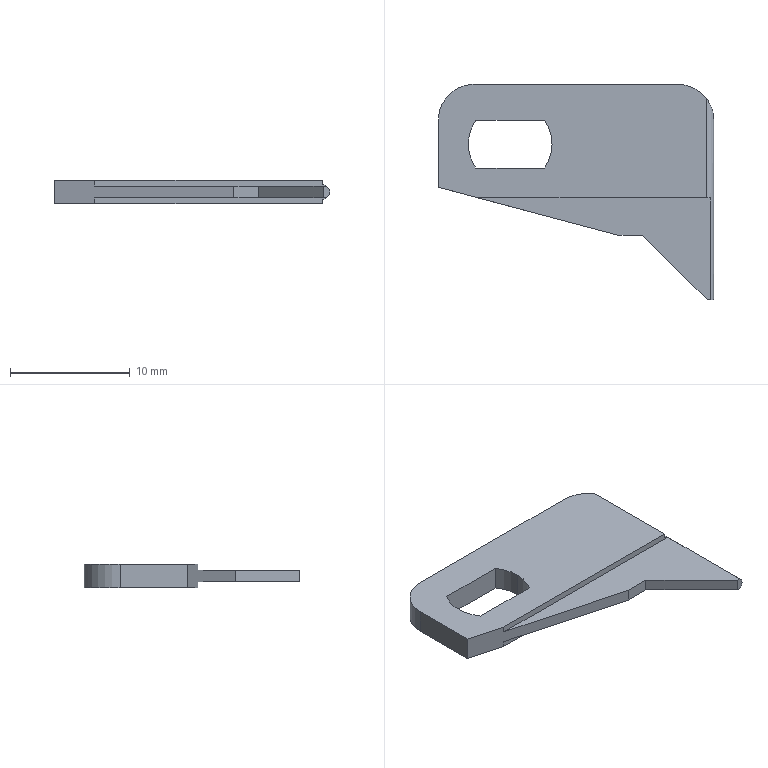Part | NX | 1 solid | 23 faces | box 23 x 18 x 2 mm | volume 428.306 mm3 | plane 16 | cylinder 7 | commonest cylinder face diameters 7 x3 1.2 x2 6 x2
STEP:
#1=CARTESIAN_POINT('',(16.4,3.8,0.));
#2=VERTEX_POINT('',#1);
#3=CARTESIAN_POINT('',(16.4,-4.5,0.));
#4=VERTEX_POINT('',#3);
#5=CARTESIAN_POINT('',(16.4,3.8,0.));
#6=DIRECTION('',(0.,-1.,0.));
#7=VECTOR('',#6,1000.);
#8=LINE('',#5,#7);
#9=EDGE_CURVE('',#2,#4,#8,.T.);
#10=ORIENTED_EDGE('',*,*,#9,.T.);
#11=CARTESIAN_POINT('',(-2.625,-4.5,0.));
#12=VERTEX_POINT('',#11);
#13=CARTESIAN_POINT('',(16.4,-4.5,0.));
#14=DIRECTION('',(-1.,0.,0.));
#15=VECTOR('',#14,1000.);
#16=LINE('',#13,#15);
#17=EDGE_CURVE('',#4,#12,#16,.T.);
#18=ORIENTED_EDGE('',*,*,#17,.T.);
#19=CARTESIAN_POINT('',(-6.,-3.6,0.));
#20=VERTEX_POINT('',#19);
#21=CARTESIAN_POINT('',(-6.,-3.6,0.));
#22=DIRECTION('',(0.9662,-0.2577,0.));
#23=VECTOR('',#22,1000.);
#24=LINE('',#21,#23);
#25=EDGE_CURVE('',#20,#12,#24,.T.);
#26=ORIENTED_EDGE('',*,*,#25,.F.);
#27=CARTESIAN_POINT('',(-6.,2.,0.));
#28=VERTEX_POINT('',#27);
#29=CARTESIAN_POINT('',(-6.,-3.6,0.));
#30=DIRECTION('',(0.,1.,0.));
#31=VECTOR('',#30,1000.);
#32=LINE('',#29,#31);
#33=EDGE_CURVE('',#20,#28,#32,.T.);
#34=ORIENTED_EDGE('',*,*,#33,.T.);
#35=CARTESIAN_POINT('',(-3.,5.,0.));
#36=VERTEX_POINT('',#35);
#37=CARTESIAN_POINT('',(-3.,2.,0.));
#38=DIRECTION('',(0.,0.,1.));
#39=DIRECTION('',(0.,1.,0.));
#40=AXIS2_PLACEMENT_3D('',#37,#38,#39);
#41=CIRCLE('',#40,3.);
#42=EDGE_CURVE('',#36,#28,#41,.T.);
#43=ORIENTED_EDGE('',*,*,#42,.F.);
#44=CARTESIAN_POINT('',(14.,5.,0.));
#45=VERTEX_POINT('',#44);
#46=CARTESIAN_POINT('',(-3.,5.,0.));
#47=DIRECTION('',(1.,0.,0.));
#48=VECTOR('',#47,1000.);
#49=LINE('',#46,#48);
#50=EDGE_CURVE('',#36,#45,#49,.T.);
#51=ORIENTED_EDGE('',*,*,#50,.T.);
#52=CARTESIAN_POINT('',(14.,2.,0.));
#53=DIRECTION('',(0.,0.,1.));
#54=DIRECTION('',(0.8,0.6,0.));
#55=AXIS2_PLACEMENT_3D('',#52,#53,#54);
#56=CIRCLE('',#55,3.);
#57=EDGE_CURVE('',#2,#45,#56,.T.);
#58=ORIENTED_EDGE('',*,*,#57,.F.);
#59=EDGE_LOOP('',(#10,#18,#26,#34,#43,#51,#58));
#60=FACE_BOUND('',#59,.T.);
#61=CARTESIAN_POINT('',(-2.872,-2.,0.));
#62=VERTEX_POINT('',#61);
#63=CARTESIAN_POINT('',(-2.872,2.,0.));
#64=VERTEX_POINT('',#63);
#65=CARTESIAN_POINT('',(0.,0.,0.));
#66=DIRECTION('',(0.,0.,-1.));
#67=DIRECTION('',(-1.,0.,0.));
#68=AXIS2_PLACEMENT_3D('',#65,#66,#67);
#69=CIRCLE('',#68,3.5);
#70=EDGE_CURVE('',#62,#64,#69,.T.);
#71=ORIENTED_EDGE('',*,*,#70,.F.);
#72=CARTESIAN_POINT('',(2.872,-2.,0.));
#73=VERTEX_POINT('',#72);
#74=CARTESIAN_POINT('',(-2.872,-2.,0.));
#75=DIRECTION('',(1.,0.,0.));
#76=VECTOR('',#75,1000.);
#77=LINE('',#74,#76);
#78=EDGE_CURVE('',#62,#73,#77,.T.);
#79=ORIENTED_EDGE('',*,*,#78,.T.);
#80=CARTESIAN_POINT('',(3.5,0.,0.));
#81=VERTEX_POINT('',#80);
#82=CARTESIAN_POINT('',(0.,0.,0.));
#83=DIRECTION('',(0.,0.,-1.));
#84=DIRECTION('',(1.,0.,0.));
#85=AXIS2_PLACEMENT_3D('',#82,#83,#84);
#86=CIRCLE('',#85,3.5);
#87=EDGE_CURVE('',#81,#73,#86,.T.);
#88=ORIENTED_EDGE('',*,*,#87,.F.);
#89=CARTESIAN_POINT('',(2.872,2.,0.));
#90=VERTEX_POINT('',#89);
#91=CARTESIAN_POINT('',(0.,0.,0.));
#92=DIRECTION('',(0.,0.,-1.));
#93=DIRECTION('',(1.,0.,0.));
#94=AXIS2_PLACEMENT_3D('',#91,#92,#93);
#95=CIRCLE('',#94,3.5);
#96=EDGE_CURVE('',#90,#81,#95,.T.);
#97=ORIENTED_EDGE('',*,*,#96,.F.);
#98=CARTESIAN_POINT('',(2.872,2.,0.));
#99=DIRECTION('',(-1.,0.,0.));
#100=VECTOR('',#99,1000.);
#101=LINE('',#98,#100);
#102=EDGE_CURVE('',#90,#64,#101,.T.);
#103=ORIENTED_EDGE('',*,*,#102,.T.);
#104=EDGE_LOOP('',(#71,#79,#88,#97,#103));
#105=FACE_BOUND('',#104,.T.);
#106=CARTESIAN_POINT('',(0.,0.,0.));
#107=DIRECTION('',(0.,0.,1.));
#108=DIRECTION('',(1.,0.,0.));
#109=AXIS2_PLACEMENT_3D('',#106,#107,#108);
#110=PLANE('',#109);
#111=ADVANCED_FACE('',(#60,#105),#110,.F.);
#112=ORIENTED_EDGE('',*,*,#9,.F.);
#113=CARTESIAN_POINT('',(16.4,3.8,0.4));
#114=VERTEX_POINT('',#113);
#115=CARTESIAN_POINT('',(16.4,3.8,0.));
#116=DIRECTION('',(0.,0.,1.));
#117=VECTOR('',#116,1000.);
#118=LINE('',#115,#117);
#119=EDGE_CURVE('',#2,#114,#118,.T.);
#120=ORIENTED_EDGE('',*,*,#119,.T.);
#121=CARTESIAN_POINT('',(16.4,-4.5,0.4));
#122=VERTEX_POINT('',#121);
#123=CARTESIAN_POINT('',(16.4,3.8,0.4));
#124=DIRECTION('',(0.,-1.,0.));
#125=VECTOR('',#124,1000.);
#126=LINE('',#123,#125);
#127=EDGE_CURVE('',#114,#122,#126,.T.);
#128=ORIENTED_EDGE('',*,*,#127,.T.);
#129=CARTESIAN_POINT('',(16.4,-4.5,0.4));
#130=DIRECTION('',(0.,0.,-1.));
#131=VECTOR('',#130,1000.);
#132=LINE('',#129,#131);
#133=EDGE_CURVE('',#122,#4,#132,.T.);
#134=ORIENTED_EDGE('',*,*,#133,.T.);
#135=EDGE_LOOP('',(#112,#120,#128,#134));
#136=FACE_BOUND('',#135,.T.);
#137=CARTESIAN_POINT('',(16.4,-13.,0.4));
#138=DIRECTION('',(-1.,0.,0.));
#139=DIRECTION('',(0.,0.,1.));
#140=AXIS2_PLACEMENT_3D('',#137,#138,#139);
#141=PLANE('',#140);
#142=ADVANCED_FACE('',(#136),#141,.F.);
#143=CARTESIAN_POINT('',(16.732,-4.5,0.5));
#144=VERTEX_POINT('',#143);
#145=CARTESIAN_POINT('',(-2.625,-4.5,0.5));
#146=VERTEX_POINT('',#145);
#147=CARTESIAN_POINT('',(16.732,-4.5,0.5));
#148=DIRECTION('',(-1.,0.,0.));
#149=VECTOR('',#148,1000.);
#150=LINE('',#147,#149);
#151=EDGE_CURVE('',#144,#146,#150,.T.);
#152=ORIENTED_EDGE('',*,*,#151,.T.);
#153=CARTESIAN_POINT('',(-2.625,-4.5,0.5));
#154=DIRECTION('',(0.,0.,-1.));
#155=VECTOR('',#154,1000.);
#156=LINE('',#153,#155);
#157=EDGE_CURVE('',#146,#12,#156,.T.);
#158=ORIENTED_EDGE('',*,*,#157,.T.);
#159=ORIENTED_EDGE('',*,*,#17,.F.);
#160=ORIENTED_EDGE('',*,*,#133,.F.);
#161=CARTESIAN_POINT('',(16.4,-4.5,1.));
#162=DIRECTION('',(0.,1.,0.));
#163=DIRECTION('',(0.5528,0.,-0.8333));
#164=AXIS2_PLACEMENT_3D('',#161,#162,#163);
#165=CIRCLE('',#164,0.6);
#166=EDGE_CURVE('',#144,#122,#165,.T.);
#167=ORIENTED_EDGE('',*,*,#166,.F.);
#168=EDGE_LOOP('',(#152,#158,#159,#160,#167));
#169=FACE_BOUND('',#168,.T.);
#170=CARTESIAN_POINT('',(-6.,-4.5,0.5));
#171=DIRECTION('',(0.,1.,0.));
#172=DIRECTION('',(1.,0.,0.));
#173=AXIS2_PLACEMENT_3D('',#170,#171,#172);
#174=PLANE('',#173);
#175=ADVANCED_FACE('',(#169),#174,.F.);
#176=CARTESIAN_POINT('',(16.732,-13.,0.5));
#177=VERTEX_POINT('',#176);
#178=CARTESIAN_POINT('',(16.732,-4.5,0.5));
#179=DIRECTION('',(0.,-1.,0.));
#180=VECTOR('',#179,1000.);
#181=LINE('',#178,#180);
#182=EDGE_CURVE('',#144,#177,#181,.T.);
#183=ORIENTED_EDGE('',*,*,#182,.T.);
#184=CARTESIAN_POINT('',(16.45,-13.,0.5));
#185=VERTEX_POINT('',#184);
#186=CARTESIAN_POINT('',(16.732,-13.,0.5));
#187=DIRECTION('',(-1.,0.,0.));
#188=VECTOR('',#187,1000.);
#189=LINE('',#186,#188);
#190=EDGE_CURVE('',#177,#185,#189,.T.);
#191=ORIENTED_EDGE('',*,*,#190,.T.);
#192=CARTESIAN_POINT('',(11.05,-7.6,0.5));
#193=VERTEX_POINT('',#192);
#194=CARTESIAN_POINT('',(11.05,-7.6,0.5));
#195=DIRECTION('',(0.7071,-0.7071,0.));
#196=VECTOR('',#195,1000.);
#197=LINE('',#194,#196);
#198=EDGE_CURVE('',#193,#185,#197,.T.);
#199=ORIENTED_EDGE('',*,*,#198,.F.);
#200=CARTESIAN_POINT('',(9.,-7.6,0.5));
#201=VERTEX_POINT('',#200);
#202=CARTESIAN_POINT('',(11.05,-7.6,0.5));
#203=DIRECTION('',(-1.,0.,0.));
#204=VECTOR('',#203,1000.);
#205=LINE('',#202,#204);
#206=EDGE_CURVE('',#193,#201,#205,.T.);
#207=ORIENTED_EDGE('',*,*,#206,.T.);
#208=CARTESIAN_POINT('',(-2.625,-4.5,0.5));
#209=DIRECTION('',(0.9662,-0.2577,0.));
#210=VECTOR('',#209,1000.);
#211=LINE('',#208,#210);
#212=EDGE_CURVE('',#146,#201,#211,.T.);
#213=ORIENTED_EDGE('',*,*,#212,.F.);
#214=ORIENTED_EDGE('',*,*,#151,.F.);
#215=EDGE_LOOP('',(#183,#191,#199,#207,#213,#214));
#216=FACE_BOUND('',#215,.T.);
#217=CARTESIAN_POINT('',(-6.,-13.,0.5));
#218=DIRECTION('',(0.,0.,1.));
#219=DIRECTION('',(1.,0.,0.));
#220=AXIS2_PLACEMENT_3D('',#217,#218,#219);
#221=PLANE('',#220);
#222=ADVANCED_FACE('',(#216),#221,.F.);
#223=CARTESIAN_POINT('',(17.,2.,1.));
#224=VERTEX_POINT('',#223);
#225=CARTESIAN_POINT('',(17.,-13.,1.));
#226=VERTEX_POINT('',#225);
#227=CARTESIAN_POINT('',(17.,-13.,1.));
#228=DIRECTION('',(0.,-1.,0.));
#229=VECTOR('',#228,1000.);
#230=LINE('',#227,#229);
#231=EDGE_CURVE('',#224,#226,#230,.T.);
#232=ORIENTED_EDGE('',*,*,#231,.F.);
#233=CARTESIAN_POINT('',(16.4,3.8,1.6));
#234=VERTEX_POINT('',#233);
#235=CARTESIAN_POINT('',(17.,2.,1.));
#236=CARTESIAN_POINT('',(17.,2.241,1.108));
#237=CARTESIAN_POINT('',(16.937,2.669,1.297));
#238=CARTESIAN_POINT('',(16.788,3.166,1.49));
#239=CARTESIAN_POINT('',(16.542,3.61,1.6));
#240=CARTESIAN_POINT('',(16.4,3.8,1.6));
#241=B_SPLINE_CURVE_WITH_KNOTS('',3,(#235,#236,#237,#238,#239,#240),.UNSPECIFIED.,.F.,.F.,(4,1,1,4),(0.,0.25,0.5,1.),.UNSPECIFIED.);
#242=EDGE_CURVE('',#224,#234,#241,.T.);
#243=ORIENTED_EDGE('',*,*,#242,.T.);
#244=CARTESIAN_POINT('',(16.4,-4.5,1.6));
#245=VERTEX_POINT('',#244);
#246=CARTESIAN_POINT('',(16.4,-4.5,1.6));
#247=DIRECTION('',(0.,1.,0.));
#248=VECTOR('',#247,1000.);
#249=LINE('',#246,#248);
#250=EDGE_CURVE('',#245,#234,#249,.T.);
#251=ORIENTED_EDGE('',*,*,#250,.F.);
#252=CARTESIAN_POINT('',(16.732,-4.5,1.5));
#253=VERTEX_POINT('',#252);
#254=CARTESIAN_POINT('',(16.4,-4.5,1.));
#255=DIRECTION('',(0.,1.,0.));
#256=DIRECTION('',(0.,0.,1.));
#257=AXIS2_PLACEMENT_3D('',#254,#255,#256);
#258=CIRCLE('',#257,0.6);
#259=EDGE_CURVE('',#245,#253,#258,.T.);
#260=ORIENTED_EDGE('',*,*,#259,.T.);
#261=CARTESIAN_POINT('',(16.732,-13.,1.5));
#262=VERTEX_POINT('',#261);
#263=CARTESIAN_POINT('',(16.732,-13.,1.5));
#264=DIRECTION('',(0.,1.,0.));
#265=VECTOR('',#264,1000.);
#266=LINE('',#263,#265);
#267=EDGE_CURVE('',#262,#253,#266,.T.);
#268=ORIENTED_EDGE('',*,*,#267,.F.);
#269=CARTESIAN_POINT('',(16.4,-13.,1.));
#270=DIRECTION('',(0.,1.,0.));
#271=DIRECTION('',(0.5528,0.,0.8333));
#272=AXIS2_PLACEMENT_3D('',#269,#270,#271);
#273=CIRCLE('',#272,0.6);
#274=EDGE_CURVE('',#262,#226,#273,.T.);
#275=ORIENTED_EDGE('',*,*,#274,.T.);
#276=EDGE_LOOP('',(#232,#243,#251,#260,#268,#275));
#277=FACE_BOUND('',#276,.T.);
#278=CARTESIAN_POINT('',(16.4,-13.,1.));
#279=DIRECTION('',(0.,-1.,0.));
#280=DIRECTION('',(1.,0.,0.));
#281=AXIS2_PLACEMENT_3D('',#278,#279,#280);
#282=CYLINDRICAL_SURFACE('',#281,0.6);
#283=ADVANCED_FACE('',(#277),#282,.T.);
#284=ORIENTED_EDGE('',*,*,#274,.F.);
#285=CARTESIAN_POINT('',(16.45,-13.,1.5));
#286=VERTEX_POINT('',#285);
#287=CARTESIAN_POINT('',(16.732,-13.,1.5));
#288=DIRECTION('',(-1.,0.,0.));
#289=VECTOR('',#288,1000.);
#290=LINE('',#287,#289);
#291=EDGE_CURVE('',#262,#286,#290,.T.);
#292=ORIENTED_EDGE('',*,*,#291,.T.);
#293=CARTESIAN_POINT('',(16.45,-13.,1.5));
#294=DIRECTION('',(0.,0.,-1.));
#295=VECTOR('',#294,1000.);
#296=LINE('',#293,#295);
#297=EDGE_CURVE('',#286,#185,#296,.T.);
#298=ORIENTED_EDGE('',*,*,#297,.T.);
#299=ORIENTED_EDGE('',*,*,#190,.F.);
#300=CARTESIAN_POINT('',(16.4,-13.,1.));
#301=DIRECTION('',(0.,1.,0.));
#302=DIRECTION('',(0.5528,0.,0.8333));
#303=AXIS2_PLACEMENT_3D('',#300,#301,#302);
#304=CIRCLE('',#303,0.6);
#305=EDGE_CURVE('',#226,#177,#304,.T.);
#306=ORIENTED_EDGE('',*,*,#305,.F.);
#307=EDGE_LOOP('',(#284,#292,#298,#299,#306));
#308=FACE_BOUND('',#307,.T.);
#309=CARTESIAN_POINT('',(16.45,-13.,0.));
#310=DIRECTION('',(0.,-1.,0.));
#311=DIRECTION('',(0.,0.,-1.));
#312=AXIS2_PLACEMENT_3D('',#309,#310,#311);
#313=PLANE('',#312);
#314=ADVANCED_FACE('',(#308),#313,.T.);
#315=ORIENTED_EDGE('',*,*,#198,.T.);
#316=ORIENTED_EDGE('',*,*,#297,.F.);
#317=CARTESIAN_POINT('',(11.05,-7.6,1.5));
#318=VERTEX_POINT('',#317);
#319=CARTESIAN_POINT('',(16.45,-13.,1.5));
#320=DIRECTION('',(-0.7071,0.7071,0.));
#321=VECTOR('',#320,1000.);
#322=LINE('',#319,#321);
#323=EDGE_CURVE('',#286,#318,#322,.T.);
#324=ORIENTED_EDGE('',*,*,#323,.T.);
#325=CARTESIAN_POINT('',(11.05,-7.6,1.5));
#326=DIRECTION('',(0.,0.,-1.));
#327=VECTOR('',#326,1000.);
#328=LINE('',#325,#327);
#329=EDGE_CURVE('',#318,#193,#328,.T.);
#330=ORIENTED_EDGE('',*,*,#329,.T.);
#331=EDGE_LOOP('',(#315,#316,#324,#330));
#332=FACE_BOUND('',#331,.T.);
#333=CARTESIAN_POINT('',(11.05,-7.6,0.));
#334=DIRECTION('',(-0.7071,-0.7071,0.));
#335=DIRECTION('',(-0.7071,0.7071,0.));
#336=AXIS2_PLACEMENT_3D('',#333,#334,#335);
#337=PLANE('',#336);
#338=ADVANCED_FACE('',(#332),#337,.T.);
#339=ORIENTED_EDGE('',*,*,#206,.F.);
#340=ORIENTED_EDGE('',*,*,#329,.F.);
#341=CARTESIAN_POINT('',(9.,-7.6,1.5));
#342=VERTEX_POINT('',#341);
#343=CARTESIAN_POINT('',(11.05,-7.6,1.5));
#344=DIRECTION('',(-1.,0.,0.));
#345=VECTOR('',#344,1000.);
#346=LINE('',#343,#345);
#347=EDGE_CURVE('',#318,#342,#346,.T.);
#348=ORIENTED_EDGE('',*,*,#347,.T.);
#349=CARTESIAN_POINT('',(9.,-7.6,1.5));
#350=DIRECTION('',(0.,0.,-1.));
#351=VECTOR('',#350,1000.);
#352=LINE('',#349,#351);
#353=EDGE_CURVE('',#342,#201,#352,.T.);
#354=ORIENTED_EDGE('',*,*,#353,.T.);
#355=EDGE_LOOP('',(#339,#340,#348,#354));
#356=FACE_BOUND('',#355,.T.);
#357=CARTESIAN_POINT('',(-3.,-7.6,0.));
#358=DIRECTION('',(0.,-1.,0.));
#359=DIRECTION('',(0.,0.,-1.));
#360=AXIS2_PLACEMENT_3D('',#357,#358,#359);
#361=PLANE('',#360);
#362=ADVANCED_FACE('',(#356),#361,.T.);
#363=ORIENTED_EDGE('',*,*,#212,.T.);
#364=ORIENTED_EDGE('',*,*,#353,.F.);
#365=CARTESIAN_POINT('',(-2.625,-4.5,1.5));
#366=VERTEX_POINT('',#365);
#367=CARTESIAN_POINT('',(9.,-7.6,1.5));
#368=DIRECTION('',(-0.9662,0.2577,0.));
#369=VECTOR('',#368,1000.);
#370=LINE('',#367,#369);
#371=EDGE_CURVE('',#342,#366,#370,.T.);
#372=ORIENTED_EDGE('',*,*,#371,.T.);
#373=CARTESIAN_POINT('',(-2.625,-4.5,2.));
#374=VERTEX_POINT('',#373);
#375=CARTESIAN_POINT('',(-2.625,-4.5,1.5));
#376=DIRECTION('',(0.,0.,1.));
#377=VECTOR('',#376,1000.);
#378=LINE('',#375,#377);
#379=EDGE_CURVE('',#366,#374,#378,.T.);
#380=ORIENTED_EDGE('',*,*,#379,.T.);
#381=CARTESIAN_POINT('',(-6.,-3.6,2.));
#382=VERTEX_POINT('',#381);
#383=CARTESIAN_POINT('',(-2.625,-4.5,2.));
#384=DIRECTION('',(-0.9662,0.2577,0.));
#385=VECTOR('',#384,1000.);
#386=LINE('',#383,#385);
#387=EDGE_CURVE('',#374,#382,#386,.T.);
#388=ORIENTED_EDGE('',*,*,#387,.T.);
#389=CARTESIAN_POINT('',(-6.,-3.6,2.));
#390=DIRECTION('',(0.,0.,-1.));
#391=VECTOR('',#390,1000.);
#392=LINE('',#389,#391);
#393=EDGE_CURVE('',#382,#20,#392,.T.);
#394=ORIENTED_EDGE('',*,*,#393,.T.);
#395=ORIENTED_EDGE('',*,*,#25,.T.);
#396=ORIENTED_EDGE('',*,*,#157,.F.);
#397=EDGE_LOOP('',(#363,#364,#372,#380,#388,#394,#395,#396));
#398=FACE_BOUND('',#397,.T.);
#399=CARTESIAN_POINT('',(-6.,-3.6,0.));
#400=DIRECTION('',(0.2577,0.9662,0.));
#401=DIRECTION('',(0.,0.,-1.));
#402=AXIS2_PLACEMENT_3D('',#399,#400,#401);
#403=PLANE('',#402);
#404=ADVANCED_FACE('',(#398),#403,.F.);
#405=ORIENTED_EDGE('',*,*,#393,.F.);
#406=CARTESIAN_POINT('',(-6.,2.,2.));
#407=VERTEX_POINT('',#406);
#408=CARTESIAN_POINT('',(-6.,-3.6,2.));
#409=DIRECTION('',(0.,1.,0.));
#410=VECTOR('',#409,1000.);
#411=LINE('',#408,#410);
#412=EDGE_CURVE('',#382,#407,#411,.T.);
#413=ORIENTED_EDGE('',*,*,#412,.T.);
#414=CARTESIAN_POINT('',(-6.,2.,0.));
#415=DIRECTION('',(0.,0.,1.));
#416=VECTOR('',#415,1000.);
#417=LINE('',#414,#416);
#418=EDGE_CURVE('',#28,#407,#417,.T.);
#419=ORIENTED_EDGE('',*,*,#418,.F.);
#420=ORIENTED_EDGE('',*,*,#33,.F.);
#421=EDGE_LOOP('',(#405,#413,#419,#420));
#422=FACE_BOUND('',#421,.T.);
#423=CARTESIAN_POINT('',(-6.,2.,0.));
#424=DIRECTION('',(-1.,0.,0.));
#425=DIRECTION('',(0.,0.,1.));
#426=AXIS2_PLACEMENT_3D('',#423,#424,#425);
#427=PLANE('',#426);
#428=ADVANCED_FACE('',(#422),#427,.T.);
#429=ORIENTED_EDGE('',*,*,#42,.T.);
#430=ORIENTED_EDGE('',*,*,#418,.T.);
#431=CARTESIAN_POINT('',(-3.,5.,2.));
#432=VERTEX_POINT('',#431);
#433=CARTESIAN_POINT('',(-3.,2.,2.));
#434=DIRECTION('',(0.,0.,-1.));
#435=DIRECTION('',(-1.,0.,0.));
#436=AXIS2_PLACEMENT_3D('',#433,#434,#435);
#437=CIRCLE('',#436,3.);
#438=EDGE_CURVE('',#407,#432,#437,.T.);
#439=ORIENTED_EDGE('',*,*,#438,.T.);
#440=CARTESIAN_POINT('',(-3.,5.,0.));
#441=DIRECTION('',(0.,0.,1.));
#442=VECTOR('',#441,1000.);
#443=LINE('',#440,#442);
#444=EDGE_CURVE('',#36,#432,#443,.T.);
#445=ORIENTED_EDGE('',*,*,#444,.F.);
#446=EDGE_LOOP('',(#429,#430,#439,#445));
#447=FACE_BOUND('',#446,.T.);
#448=CARTESIAN_POINT('',(-3.,2.,0.));
#449=DIRECTION('',(0.,0.,1.));
#450=DIRECTION('',(1.,0.,0.));
#451=AXIS2_PLACEMENT_3D('',#448,#449,#450);
#452=CYLINDRICAL_SURFACE('',#451,3.);
#453=ADVANCED_FACE('',(#447),#452,.T.);
#454=ORIENTED_EDGE('',*,*,#50,.F.);
#455=ORIENTED_EDGE('',*,*,#444,.T.);
#456=CARTESIAN_POINT('',(14.,5.,2.));
#457=VERTEX_POINT('',#456);
#458=CARTESIAN_POINT('',(-3.,5.,2.));
#459=DIRECTION('',(1.,0.,0.));
#460=VECTOR('',#459,1000.);
#461=LINE('',#458,#460);
#462=EDGE_CURVE('',#432,#457,#461,.T.);
#463=ORIENTED_EDGE('',*,*,#462,.T.);
#464=CARTESIAN_POINT('',(14.,5.,2.));
#465=DIRECTION('',(0.,0.,-1.));
#466=VECTOR('',#465,1000.);
#467=LINE('',#464,#466);
#468=EDGE_CURVE('',#457,#45,#467,.T.);
#469=ORIENTED_EDGE('',*,*,#468,.T.);
#470=EDGE_LOOP('',(#454,#455,#463,#469));
#471=FACE_BOUND('',#470,.T.);
#472=CARTESIAN_POINT('',(14.,5.,0.));
#473=DIRECTION('',(0.,1.,0.));
#474=DIRECTION('',(1.,0.,0.));
#475=AXIS2_PLACEMENT_3D('',#472,#473,#474);
#476=PLANE('',#475);
#477=ADVANCED_FACE('',(#471),#476,.T.);
#478=CARTESIAN_POINT('',(16.4,3.8,2.));
#479=VERTEX_POINT('',#478);
#480=CARTESIAN_POINT('',(16.4,3.8,1.6));
#481=DIRECTION('',(0.,0.,1.));
#482=VECTOR('',#481,1000.);
#483=LINE('',#480,#482);
#484=EDGE_CURVE('',#234,#479,#483,.T.);
#485=ORIENTED_EDGE('',*,*,#484,.F.);
#486=ORIENTED_EDGE('',*,*,#242,.F.);
#487=CARTESIAN_POINT('',(17.,2.,1.));
#488=CARTESIAN_POINT('',(17.,2.257,0.8849));
#489=CARTESIAN_POINT('',(16.961,2.556,0.7511));
#490=CARTESIAN_POINT('',(16.75,3.295,0.46));
#491=CARTESIAN_POINT('',(16.54,3.613,0.4));
#492=CARTESIAN_POINT('',(16.4,3.8,0.4));
#493=B_SPLINE_CURVE_WITH_KNOTS('',3,(#487,#488,#489,#490,#491,#492),.UNSPECIFIED.,.F.,.F.,(4,1,1,4),(0.,0.25,0.5,1.),.UNSPECIFIED.);
#494=EDGE_CURVE('',#114,#224,#493,.F.);
#495=ORIENTED_EDGE('',*,*,#494,.F.);
#496=ORIENTED_EDGE('',*,*,#119,.F.);
#497=ORIENTED_EDGE('',*,*,#57,.T.);
#498=ORIENTED_EDGE('',*,*,#468,.F.);
#499=CARTESIAN_POINT('',(14.,2.,2.));
#500=DIRECTION('',(0.,0.,-1.));
#501=DIRECTION('',(0.,1.,0.));
#502=AXIS2_PLACEMENT_3D('',#499,#500,#501);
#503=CIRCLE('',#502,3.);
#504=EDGE_CURVE('',#457,#479,#503,.T.);
#505=ORIENTED_EDGE('',*,*,#504,.T.);
#506=EDGE_LOOP('',(#485,#486,#495,#496,#497,#498,#505));
#507=FACE_BOUND('',#506,.T.);
#508=CARTESIAN_POINT('',(14.,2.,0.));
#509=DIRECTION('',(0.,0.,1.));
#510=DIRECTION('',(1.,0.,0.));
#511=AXIS2_PLACEMENT_3D('',#508,#509,#510);
#512=CYLINDRICAL_SURFACE('',#511,3.);
#513=ADVANCED_FACE('',(#507),#512,.T.);
#514=CARTESIAN_POINT('',(16.4,-4.5,2.));
#515=VERTEX_POINT('',#514);
#516=CARTESIAN_POINT('',(16.4,3.8,2.));
#517=DIRECTION('',(0.,-1.,0.));
#518=VECTOR('',#517,1000.);
#519=LINE('',#516,#518);
#520=EDGE_CURVE('',#479,#515,#519,.T.);
#521=ORIENTED_EDGE('',*,*,#520,.T.);
#522=CARTESIAN_POINT('',(16.4,-4.5,1.6));
#523=DIRECTION('',(0.,0.,1.));
#524=VECTOR('',#523,1000.);
#525=LINE('',#522,#524);
#526=EDGE_CURVE('',#245,#515,#525,.T.);
#527=ORIENTED_EDGE('',*,*,#526,.F.);
#528=ORIENTED_EDGE('',*,*,#250,.T.);
#529=ORIENTED_EDGE('',*,*,#484,.T.);
#530=EDGE_LOOP('',(#521,#527,#528,#529));
#531=FACE_BOUND('',#530,.T.);
#532=CARTESIAN_POINT('',(16.4,-13.,2.));
#533=DIRECTION('',(-1.,0.,0.));
#534=DIRECTION('',(0.,0.,1.));
#535=AXIS2_PLACEMENT_3D('',#532,#533,#534);
#536=PLANE('',#535);
#537=ADVANCED_FACE('',(#531),#536,.F.);
#538=ORIENTED_EDGE('',*,*,#520,.F.);
#539=ORIENTED_EDGE('',*,*,#504,.F.);
#540=ORIENTED_EDGE('',*,*,#462,.F.);
#541=ORIENTED_EDGE('',*,*,#438,.F.);
#542=ORIENTED_EDGE('',*,*,#412,.F.);
#543=ORIENTED_EDGE('',*,*,#387,.F.);
#544=CARTESIAN_POINT('',(16.4,-4.5,2.));
#545=DIRECTION('',(-1.,0.,0.));
#546=VECTOR('',#545,1000.);
#547=LINE('',#544,#546);
#548=EDGE_CURVE('',#515,#374,#547,.T.);
#549=ORIENTED_EDGE('',*,*,#548,.F.);
#550=EDGE_LOOP('',(#538,#539,#540,#541,#542,#543,#549));
#551=FACE_BOUND('',#550,.T.);
#552=CARTESIAN_POINT('',(-2.872,2.,2.));
#553=VERTEX_POINT('',#552);
#554=CARTESIAN_POINT('',(-2.872,-2.,2.));
#555=VERTEX_POINT('',#554);
#556=CARTESIAN_POINT('',(0.,0.,2.));
#557=DIRECTION('',(0.,0.,1.));
#558=DIRECTION('',(-1.,0.,0.));
#559=AXIS2_PLACEMENT_3D('',#556,#557,#558);
#560=CIRCLE('',#559,3.5);
#561=EDGE_CURVE('',#553,#555,#560,.T.);
#562=ORIENTED_EDGE('',*,*,#561,.F.);
#563=CARTESIAN_POINT('',(2.872,2.,2.));
#564=VERTEX_POINT('',#563);
#565=CARTESIAN_POINT('',(2.872,2.,2.));
#566=DIRECTION('',(-1.,0.,0.));
#567=VECTOR('',#566,1000.);
#568=LINE('',#565,#567);
#569=EDGE_CURVE('',#564,#553,#568,.T.);
#570=ORIENTED_EDGE('',*,*,#569,.F.);
#571=CARTESIAN_POINT('',(3.5,0.,2.));
#572=VERTEX_POINT('',#571);
#573=CARTESIAN_POINT('',(0.,0.,2.));
#574=DIRECTION('',(0.,0.,1.));
#575=DIRECTION('',(1.,0.,0.));
#576=AXIS2_PLACEMENT_3D('',#573,#574,#575);
#577=CIRCLE('',#576,3.5);
#578=EDGE_CURVE('',#572,#564,#577,.T.);
#579=ORIENTED_EDGE('',*,*,#578,.F.);
#580=CARTESIAN_POINT('',(2.872,-2.,2.));
#581=VERTEX_POINT('',#580);
#582=CARTESIAN_POINT('',(0.,0.,2.));
#583=DIRECTION('',(0.,0.,1.));
#584=DIRECTION('',(1.,0.,0.));
#585=AXIS2_PLACEMENT_3D('',#582,#583,#584);
#586=CIRCLE('',#585,3.5);
#587=EDGE_CURVE('',#581,#572,#586,.T.);
#588=ORIENTED_EDGE('',*,*,#587,.F.);
#589=CARTESIAN_POINT('',(-2.872,-2.,2.));
#590=DIRECTION('',(1.,0.,0.));
#591=VECTOR('',#590,1000.);
#592=LINE('',#589,#591);
#593=EDGE_CURVE('',#555,#581,#592,.T.);
#594=ORIENTED_EDGE('',*,*,#593,.F.);
#595=EDGE_LOOP('',(#562,#570,#579,#588,#594));
#596=FACE_BOUND('',#595,.T.);
#597=CARTESIAN_POINT('',(0.,0.,2.));
#598=DIRECTION('',(0.,0.,1.));
#599=DIRECTION('',(1.,0.,0.));
#600=AXIS2_PLACEMENT_3D('',#597,#598,#599);
#601=PLANE('',#600);
#602=ADVANCED_FACE('',(#551,#596),#601,.T.);
#603=CARTESIAN_POINT('',(16.732,-4.5,1.5));
#604=DIRECTION('',(-1.,0.,0.));
#605=VECTOR('',#604,1000.);
#606=LINE('',#603,#605);
#607=EDGE_CURVE('',#253,#366,#606,.T.);
#608=ORIENTED_EDGE('',*,*,#607,.F.);
#609=ORIENTED_EDGE('',*,*,#259,.F.);
#610=ORIENTED_EDGE('',*,*,#526,.T.);
#611=ORIENTED_EDGE('',*,*,#548,.T.);
#612=ORIENTED_EDGE('',*,*,#379,.F.);
#613=EDGE_LOOP('',(#608,#609,#610,#611,#612));
#614=FACE_BOUND('',#613,.T.);
#615=CARTESIAN_POINT('',(-6.,-4.5,2.));
#616=DIRECTION('',(0.,1.,0.));
#617=DIRECTION('',(1.,0.,0.));
#618=AXIS2_PLACEMENT_3D('',#615,#616,#617);
#619=PLANE('',#618);
#620=ADVANCED_FACE('',(#614),#619,.F.);
#621=ORIENTED_EDGE('',*,*,#267,.T.);
#622=ORIENTED_EDGE('',*,*,#607,.T.);
#623=ORIENTED_EDGE('',*,*,#371,.F.);
#624=ORIENTED_EDGE('',*,*,#347,.F.);
#625=ORIENTED_EDGE('',*,*,#323,.F.);
#626=ORIENTED_EDGE('',*,*,#291,.F.);
#627=EDGE_LOOP('',(#621,#622,#623,#624,#625,#626));
#628=FACE_BOUND('',#627,.T.);
#629=CARTESIAN_POINT('',(-6.,-4.5,1.5));
#630=DIRECTION('',(0.,0.,-1.));
#631=DIRECTION('',(0.,-1.,0.));
#632=AXIS2_PLACEMENT_3D('',#629,#630,#631);
#633=PLANE('',#632);
#634=ADVANCED_FACE('',(#628),#633,.F.);
#635=ORIENTED_EDGE('',*,*,#70,.T.);
#636=CARTESIAN_POINT('',(-2.872,2.,2.));
#637=DIRECTION('',(0.,0.,-1.));
#638=VECTOR('',#637,1000.);
#639=LINE('',#636,#638);
#640=EDGE_CURVE('',#553,#64,#639,.T.);
#641=ORIENTED_EDGE('',*,*,#640,.F.);
#642=ORIENTED_EDGE('',*,*,#561,.T.);
#643=CARTESIAN_POINT('',(-2.872,-2.,0.));
#644=DIRECTION('',(0.,0.,1.));
#645=VECTOR('',#644,1000.);
#646=LINE('',#643,#645);
#647=EDGE_CURVE('',#62,#555,#646,.T.);
#648=ORIENTED_EDGE('',*,*,#647,.F.);
#649=EDGE_LOOP('',(#635,#641,#642,#648));
#650=FACE_BOUND('',#649,.T.);
#651=CARTESIAN_POINT('',(0.,0.,0.));
#652=DIRECTION('',(0.,0.,1.));
#653=DIRECTION('',(1.,0.,0.));
#654=AXIS2_PLACEMENT_3D('',#651,#652,#653);
#655=CYLINDRICAL_SURFACE('',#654,3.5);
#656=ADVANCED_FACE('',(#650),#655,.F.);
#657=ORIENTED_EDGE('',*,*,#78,.F.);
#658=ORIENTED_EDGE('',*,*,#647,.T.);
#659=ORIENTED_EDGE('',*,*,#593,.T.);
#660=CARTESIAN_POINT('',(2.872,-2.,2.));
#661=DIRECTION('',(0.,0.,-1.));
#662=VECTOR('',#661,1000.);
#663=LINE('',#660,#662);
#664=EDGE_CURVE('',#581,#73,#663,.T.);
#665=ORIENTED_EDGE('',*,*,#664,.T.);
#666=EDGE_LOOP('',(#657,#658,#659,#665));
#667=FACE_BOUND('',#666,.T.);
#668=CARTESIAN_POINT('',(2.872,-2.,0.));
#669=DIRECTION('',(0.,1.,0.));
#670=DIRECTION('',(1.,0.,0.));
#671=AXIS2_PLACEMENT_3D('',#668,#669,#670);
#672=PLANE('',#671);
#673=ADVANCED_FACE('',(#667),#672,.T.);
#674=CARTESIAN_POINT('',(3.5,0.,0.));
#675=DIRECTION('',(0.,0.,1.));
#676=VECTOR('',#675,1000.);
#677=LINE('',#674,#676);
#678=EDGE_CURVE('',#81,#572,#677,.T.);
#679=ORIENTED_EDGE('',*,*,#678,.F.);
#680=ORIENTED_EDGE('',*,*,#87,.T.);
#681=ORIENTED_EDGE('',*,*,#664,.F.);
#682=ORIENTED_EDGE('',*,*,#587,.T.);
#683=EDGE_LOOP('',(#679,#680,#681,#682));
#684=FACE_BOUND('',#683,.T.);
#685=CARTESIAN_POINT('',(0.,0.,0.));
#686=DIRECTION('',(0.,0.,1.));
#687=DIRECTION('',(1.,0.,0.));
#688=AXIS2_PLACEMENT_3D('',#685,#686,#687);
#689=CYLINDRICAL_SURFACE('',#688,3.5);
#690=ADVANCED_FACE('',(#684),#689,.F.);
#691=ORIENTED_EDGE('',*,*,#102,.F.);
#692=CARTESIAN_POINT('',(2.872,2.,0.));
#693=DIRECTION('',(0.,0.,1.));
#694=VECTOR('',#693,1000.);
#695=LINE('',#692,#694);
#696=EDGE_CURVE('',#90,#564,#695,.T.);
#697=ORIENTED_EDGE('',*,*,#696,.T.);
#698=ORIENTED_EDGE('',*,*,#569,.T.);
#699=ORIENTED_EDGE('',*,*,#640,.T.);
#700=EDGE_LOOP('',(#691,#697,#698,#699));
#701=FACE_BOUND('',#700,.T.);
#702=CARTESIAN_POINT('',(-2.872,2.,0.));
#703=DIRECTION('',(0.,-1.,0.));
#704=DIRECTION('',(0.,0.,-1.));
#705=AXIS2_PLACEMENT_3D('',#702,#703,#704);
#706=PLANE('',#705);
#707=ADVANCED_FACE('',(#701),#706,.T.);
#708=ORIENTED_EDGE('',*,*,#96,.T.);
#709=ORIENTED_EDGE('',*,*,#678,.T.);
#710=ORIENTED_EDGE('',*,*,#578,.T.);
#711=ORIENTED_EDGE('',*,*,#696,.F.);
#712=EDGE_LOOP('',(#708,#709,#710,#711));
#713=FACE_BOUND('',#712,.T.);
#714=CARTESIAN_POINT('',(0.,0.,0.));
#715=DIRECTION('',(0.,0.,1.));
#716=DIRECTION('',(1.,0.,0.));
#717=AXIS2_PLACEMENT_3D('',#714,#715,#716);
#718=CYLINDRICAL_SURFACE('',#717,3.5);
#719=ADVANCED_FACE('',(#713),#718,.F.);
#720=ORIENTED_EDGE('',*,*,#494,.T.);
#721=ORIENTED_EDGE('',*,*,#231,.T.);
#722=ORIENTED_EDGE('',*,*,#305,.T.);
#723=ORIENTED_EDGE('',*,*,#182,.F.);
#724=ORIENTED_EDGE('',*,*,#166,.T.);
#725=ORIENTED_EDGE('',*,*,#127,.F.);
#726=EDGE_LOOP('',(#720,#721,#722,#723,#724,#725));
#727=FACE_BOUND('',#726,.T.);
#728=CARTESIAN_POINT('',(16.4,-13.,1.));
#729=DIRECTION('',(0.,-1.,0.));
#730=DIRECTION('',(1.,0.,0.));
#731=AXIS2_PLACEMENT_3D('',#728,#729,#730);
#732=CYLINDRICAL_SURFACE('',#731,0.6);
#733=ADVANCED_FACE('',(#727),#732,.T.);
#734=CLOSED_SHELL('',(#111,#142,#175,#222,#283,#314,#338,#362,#404,#428,#453,#477,#513,#537,#602,#620,#634,#656,#673,#690,#707,#719,#733));
#735=MANIFOLD_SOLID_BREP('',#734);
#736=(LENGTH_UNIT()NAMED_UNIT(*)SI_UNIT(.MILLI.,.METRE.));
#737=UNCERTAINTY_MEASURE_WITH_UNIT(LENGTH_MEASURE(0.0508),#736,'','');
#738=(NAMED_UNIT(*)PLANE_ANGLE_UNIT()SI_UNIT($,.RADIAN.));
#739=(NAMED_UNIT(*)SI_UNIT($,.STERADIAN.)SOLID_ANGLE_UNIT());
#740=(GEOMETRIC_REPRESENTATION_CONTEXT(3)GLOBAL_UNCERTAINTY_ASSIGNED_CONTEXT((#737))GLOBAL_UNIT_ASSIGNED_CONTEXT((#736,#738,#739))REPRESENTATION_CONTEXT('',''));
#741=ADVANCED_BREP_SHAPE_REPRESENTATION('',(#735),#740);